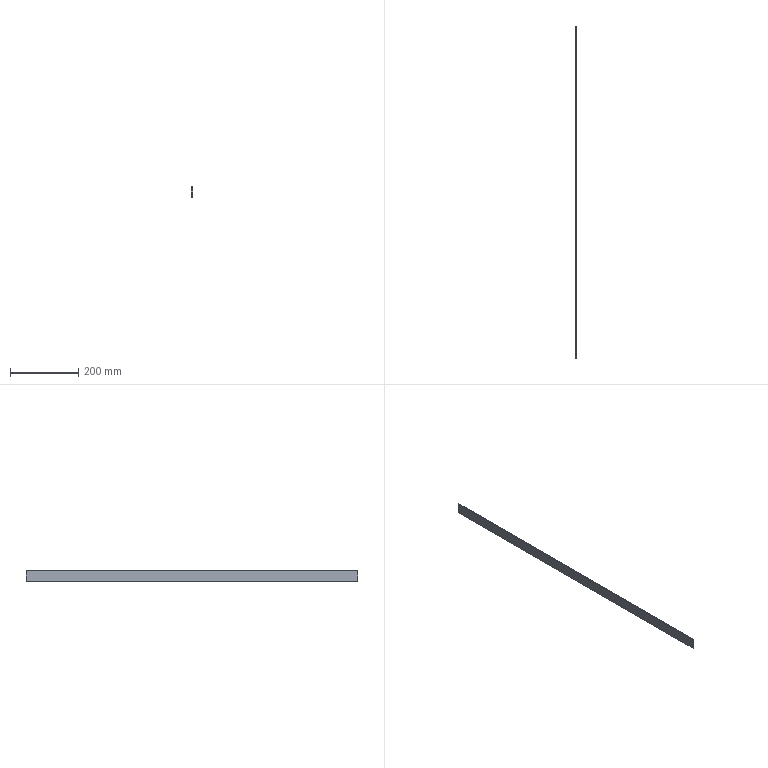Part | SolidWorks | 1 solid | 6 faces | box 3 x 970 x 30 mm | volume 87300 mm3 | plane 6
STEP:
#1=CARTESIAN_POINT('',(0.,485.,15.));
#2=VERTEX_POINT('',#1);
#3=CARTESIAN_POINT('',(0.,-485.,15.));
#4=VERTEX_POINT('',#3);
#5=CARTESIAN_POINT('',(0.,-485.,15.));
#6=DIRECTION('',(0.,-1.,0.));
#7=VECTOR('',#6,1000.);
#8=LINE('',#5,#7);
#9=EDGE_CURVE('',#2,#4,#8,.T.);
#10=ORIENTED_EDGE('',*,*,#9,.F.);
#11=CARTESIAN_POINT('',(-3.,485.,15.));
#12=VERTEX_POINT('',#11);
#13=CARTESIAN_POINT('',(-3.,485.,15.));
#14=DIRECTION('',(1.,0.,0.));
#15=VECTOR('',#14,1000.);
#16=LINE('',#13,#15);
#17=EDGE_CURVE('',#12,#2,#16,.T.);
#18=ORIENTED_EDGE('',*,*,#17,.F.);
#19=CARTESIAN_POINT('',(-3.,-485.,15.));
#20=VERTEX_POINT('',#19);
#21=CARTESIAN_POINT('',(-3.,-485.,15.));
#22=DIRECTION('',(0.,-1.,0.));
#23=VECTOR('',#22,1000.);
#24=LINE('',#21,#23);
#25=EDGE_CURVE('',#12,#20,#24,.T.);
#26=ORIENTED_EDGE('',*,*,#25,.T.);
#27=CARTESIAN_POINT('',(-3.,-485.,15.));
#28=DIRECTION('',(1.,0.,0.));
#29=VECTOR('',#28,1000.);
#30=LINE('',#27,#29);
#31=EDGE_CURVE('',#20,#4,#30,.T.);
#32=ORIENTED_EDGE('',*,*,#31,.T.);
#33=EDGE_LOOP('',(#10,#18,#26,#32));
#34=FACE_OUTER_BOUND('',#33,.T.);
#35=CARTESIAN_POINT('',(-3.,-485.,15.));
#36=DIRECTION('',(0.,0.,1.));
#37=DIRECTION('',(1.,0.,0.));
#38=AXIS2_PLACEMENT_3D('',#35,#36,#37);
#39=PLANE('',#38);
#40=ADVANCED_FACE('',(#34),#39,.T.);
#41=CARTESIAN_POINT('',(0.,485.,-15.));
#42=VERTEX_POINT('',#41);
#43=CARTESIAN_POINT('',(0.,485.,-15.));
#44=DIRECTION('',(0.,0.,1.));
#45=VECTOR('',#44,1000.);
#46=LINE('',#43,#45);
#47=EDGE_CURVE('',#42,#2,#46,.T.);
#48=ORIENTED_EDGE('',*,*,#47,.F.);
#49=CARTESIAN_POINT('',(-3.,485.,-15.));
#50=VERTEX_POINT('',#49);
#51=CARTESIAN_POINT('',(-3.,485.,-15.));
#52=DIRECTION('',(1.,0.,0.));
#53=VECTOR('',#52,1000.);
#54=LINE('',#51,#53);
#55=EDGE_CURVE('',#50,#42,#54,.T.);
#56=ORIENTED_EDGE('',*,*,#55,.F.);
#57=CARTESIAN_POINT('',(-3.,485.,-15.));
#58=DIRECTION('',(0.,0.,1.));
#59=VECTOR('',#58,1000.);
#60=LINE('',#57,#59);
#61=EDGE_CURVE('',#50,#12,#60,.T.);
#62=ORIENTED_EDGE('',*,*,#61,.T.);
#63=ORIENTED_EDGE('',*,*,#17,.T.);
#64=EDGE_LOOP('',(#48,#56,#62,#63));
#65=FACE_OUTER_BOUND('',#64,.T.);
#66=CARTESIAN_POINT('',(-3.,485.,-15.));
#67=DIRECTION('',(0.,1.,0.));
#68=DIRECTION('',(0.,0.,1.));
#69=AXIS2_PLACEMENT_3D('',#66,#67,#68);
#70=PLANE('',#69);
#71=ADVANCED_FACE('',(#65),#70,.T.);
#72=CARTESIAN_POINT('',(0.,-485.,-15.));
#73=VERTEX_POINT('',#72);
#74=CARTESIAN_POINT('',(0.,-485.,-15.));
#75=DIRECTION('',(0.,1.,0.));
#76=VECTOR('',#75,1000.);
#77=LINE('',#74,#76);
#78=EDGE_CURVE('',#73,#42,#77,.T.);
#79=ORIENTED_EDGE('',*,*,#78,.F.);
#80=CARTESIAN_POINT('',(-3.,-485.,-15.));
#81=VERTEX_POINT('',#80);
#82=CARTESIAN_POINT('',(-3.,-485.,-15.));
#83=DIRECTION('',(1.,0.,0.));
#84=VECTOR('',#83,1000.);
#85=LINE('',#82,#84);
#86=EDGE_CURVE('',#81,#73,#85,.T.);
#87=ORIENTED_EDGE('',*,*,#86,.F.);
#88=CARTESIAN_POINT('',(-3.,-485.,-15.));
#89=DIRECTION('',(0.,1.,0.));
#90=VECTOR('',#89,1000.);
#91=LINE('',#88,#90);
#92=EDGE_CURVE('',#81,#50,#91,.T.);
#93=ORIENTED_EDGE('',*,*,#92,.T.);
#94=ORIENTED_EDGE('',*,*,#55,.T.);
#95=EDGE_LOOP('',(#79,#87,#93,#94));
#96=FACE_OUTER_BOUND('',#95,.T.);
#97=CARTESIAN_POINT('',(-3.,-485.,-15.));
#98=DIRECTION('',(0.,0.,-1.));
#99=DIRECTION('',(-1.,0.,0.));
#100=AXIS2_PLACEMENT_3D('',#97,#98,#99);
#101=PLANE('',#100);
#102=ADVANCED_FACE('',(#96),#101,.T.);
#103=CARTESIAN_POINT('',(0.,-485.,-15.));
#104=DIRECTION('',(0.,0.,-1.));
#105=VECTOR('',#104,1000.);
#106=LINE('',#103,#105);
#107=EDGE_CURVE('',#4,#73,#106,.T.);
#108=ORIENTED_EDGE('',*,*,#107,.F.);
#109=ORIENTED_EDGE('',*,*,#31,.F.);
#110=CARTESIAN_POINT('',(-3.,-485.,-15.));
#111=DIRECTION('',(0.,0.,-1.));
#112=VECTOR('',#111,1000.);
#113=LINE('',#110,#112);
#114=EDGE_CURVE('',#20,#81,#113,.T.);
#115=ORIENTED_EDGE('',*,*,#114,.T.);
#116=ORIENTED_EDGE('',*,*,#86,.T.);
#117=EDGE_LOOP('',(#108,#109,#115,#116));
#118=FACE_OUTER_BOUND('',#117,.T.);
#119=CARTESIAN_POINT('',(-3.,-485.,-15.));
#120=DIRECTION('',(0.,-1.,0.));
#121=DIRECTION('',(0.,0.,-1.));
#122=AXIS2_PLACEMENT_3D('',#119,#120,#121);
#123=PLANE('',#122);
#124=ADVANCED_FACE('',(#118),#123,.T.);
#125=ORIENTED_EDGE('',*,*,#25,.F.);
#126=ORIENTED_EDGE('',*,*,#61,.F.);
#127=ORIENTED_EDGE('',*,*,#92,.F.);
#128=ORIENTED_EDGE('',*,*,#114,.F.);
#129=EDGE_LOOP('',(#125,#126,#127,#128));
#130=FACE_OUTER_BOUND('',#129,.T.);
#131=CARTESIAN_POINT('',(-3.,0.,0.));
#132=DIRECTION('',(1.,0.,0.));
#133=DIRECTION('',(0.,0.,-1.));
#134=AXIS2_PLACEMENT_3D('',#131,#132,#133);
#135=PLANE('',#134);
#136=ADVANCED_FACE('',(#130),#135,.F.);
#137=ORIENTED_EDGE('',*,*,#9,.T.);
#138=ORIENTED_EDGE('',*,*,#107,.T.);
#139=ORIENTED_EDGE('',*,*,#78,.T.);
#140=ORIENTED_EDGE('',*,*,#47,.T.);
#141=EDGE_LOOP('',(#137,#138,#139,#140));
#142=FACE_OUTER_BOUND('',#141,.T.);
#143=CARTESIAN_POINT('',(0.,0.,0.));
#144=DIRECTION('',(1.,0.,0.));
#145=DIRECTION('',(0.,0.,-1.));
#146=AXIS2_PLACEMENT_3D('',#143,#144,#145);
#147=PLANE('',#146);
#148=ADVANCED_FACE('',(#142),#147,.T.);
#149=CLOSED_SHELL('',(#40,#71,#102,#124,#136,#148));
#150=MANIFOLD_SOLID_BREP('',#149);
#151=CARTESIAN_POINT('',(0.,0.,0.));
#152=DIRECTION('',(0.,0.,1.));
#153=DIRECTION('',(1.,0.,0.));
#154=AXIS2_PLACEMENT_3D('',#151,#152,#153);
#155=(LENGTH_UNIT()NAMED_UNIT(*)SI_UNIT(.MILLI.,.METRE.));
#156=UNCERTAINTY_MEASURE_WITH_UNIT(LENGTH_MEASURE(0.00001),#155,'','');
#157=(NAMED_UNIT(*)PLANE_ANGLE_UNIT()SI_UNIT($,.RADIAN.));
#158=(NAMED_UNIT(*)SI_UNIT($,.STERADIAN.)SOLID_ANGLE_UNIT());
#159=(GEOMETRIC_REPRESENTATION_CONTEXT(3)GLOBAL_UNCERTAINTY_ASSIGNED_CONTEXT((#156))GLOBAL_UNIT_ASSIGNED_CONTEXT((#155,#157,#158))REPRESENTATION_CONTEXT('',''));
#160=ADVANCED_BREP_SHAPE_REPRESENTATION('',(#150,#154),#159);